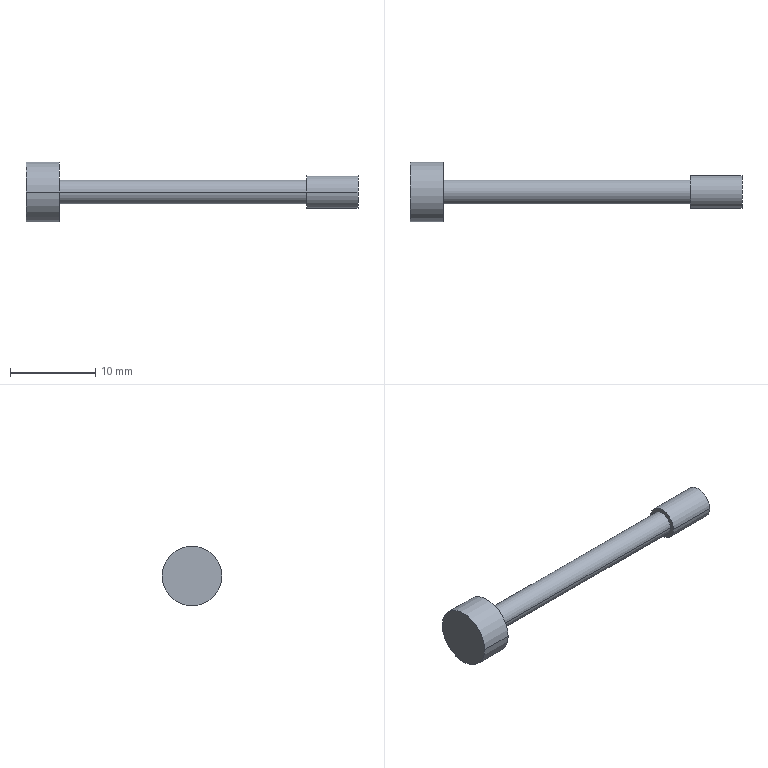Part | SolidWorks | features Revolution 1 | 1 solid | 10 faces | box 38.91 x 7 x 7 mm | volume 397.089 mm3 | cylinder 6 | plane 4 | commonest cylinder face diameters 2.8 x2 3.8 x2 7 x2
STEP:
#1=CARTESIAN_POINT('',(32.91,1.9,0.));
#2=VERTEX_POINT('',#1);
#3=CARTESIAN_POINT('',(32.91,-1.9,0.));
#4=VERTEX_POINT('',#3);
#5=CARTESIAN_POINT('',(32.91,0.,0.));
#6=DIRECTION('',(1.,0.,0.));
#7=DIRECTION('',(0.,1.,0.));
#8=AXIS2_PLACEMENT_3D('',#5,#6,#7);
#9=CIRCLE('',#8,1.9);
#10=EDGE_CURVE('',#2,#4,#9,.T.);
#11=ORIENTED_EDGE('',*,*,#10,.T.);
#12=CARTESIAN_POINT('',(38.91,-1.9,0.));
#13=VERTEX_POINT('',#12);
#14=CARTESIAN_POINT('',(38.91,-1.9,0.));
#15=DIRECTION('',(1.,0.,0.));
#16=VECTOR('',#15,1000.);
#17=LINE('',#14,#16);
#18=EDGE_CURVE('',#4,#13,#17,.T.);
#19=ORIENTED_EDGE('',*,*,#18,.T.);
#20=CARTESIAN_POINT('',(38.91,1.9,0.));
#21=VERTEX_POINT('',#20);
#22=CARTESIAN_POINT('',(38.91,0.,0.));
#23=DIRECTION('',(1.,0.,0.));
#24=DIRECTION('',(0.,1.,0.));
#25=AXIS2_PLACEMENT_3D('',#22,#23,#24);
#26=CIRCLE('',#25,1.9);
#27=EDGE_CURVE('',#21,#13,#26,.T.);
#28=ORIENTED_EDGE('',*,*,#27,.F.);
#29=CARTESIAN_POINT('',(38.91,1.9,0.));
#30=DIRECTION('',(1.,0.,0.));
#31=VECTOR('',#30,1000.);
#32=LINE('',#29,#31);
#33=EDGE_CURVE('',#2,#21,#32,.T.);
#34=ORIENTED_EDGE('',*,*,#33,.F.);
#35=EDGE_LOOP('',(#11,#19,#28,#34));
#36=FACE_OUTER_BOUND('',#35,.T.);
#37=CARTESIAN_POINT('',(38.91,0.,0.));
#38=DIRECTION('',(1.,0.,0.));
#39=DIRECTION('',(0.,1.,0.));
#40=AXIS2_PLACEMENT_3D('',#37,#38,#39);
#41=CYLINDRICAL_SURFACE('',#40,1.9);
#42=ADVANCED_FACE('',(#36),#41,.T.);
#43=CARTESIAN_POINT('',(3.91,1.4,0.));
#44=VERTEX_POINT('',#43);
#45=CARTESIAN_POINT('',(3.91,-1.4,0.));
#46=VERTEX_POINT('',#45);
#47=CARTESIAN_POINT('',(3.91,0.,0.));
#48=DIRECTION('',(1.,0.,0.));
#49=DIRECTION('',(0.,1.,0.));
#50=AXIS2_PLACEMENT_3D('',#47,#48,#49);
#51=CIRCLE('',#50,1.4);
#52=EDGE_CURVE('',#44,#46,#51,.T.);
#53=ORIENTED_EDGE('',*,*,#52,.T.);
#54=CARTESIAN_POINT('',(32.91,-1.4,0.));
#55=VERTEX_POINT('',#54);
#56=CARTESIAN_POINT('',(38.91,-1.4,0.));
#57=DIRECTION('',(1.,0.,0.));
#58=VECTOR('',#57,1000.);
#59=LINE('',#56,#58);
#60=EDGE_CURVE('',#46,#55,#59,.T.);
#61=ORIENTED_EDGE('',*,*,#60,.T.);
#62=CARTESIAN_POINT('',(32.91,1.4,0.));
#63=VERTEX_POINT('',#62);
#64=CARTESIAN_POINT('',(32.91,0.,0.));
#65=DIRECTION('',(1.,0.,0.));
#66=DIRECTION('',(0.,1.,0.));
#67=AXIS2_PLACEMENT_3D('',#64,#65,#66);
#68=CIRCLE('',#67,1.4);
#69=EDGE_CURVE('',#63,#55,#68,.T.);
#70=ORIENTED_EDGE('',*,*,#69,.F.);
#71=CARTESIAN_POINT('',(38.91,1.4,0.));
#72=DIRECTION('',(1.,0.,0.));
#73=VECTOR('',#72,1000.);
#74=LINE('',#71,#73);
#75=EDGE_CURVE('',#44,#63,#74,.T.);
#76=ORIENTED_EDGE('',*,*,#75,.F.);
#77=EDGE_LOOP('',(#53,#61,#70,#76));
#78=FACE_OUTER_BOUND('',#77,.T.);
#79=CARTESIAN_POINT('',(38.91,0.,0.));
#80=DIRECTION('',(1.,0.,0.));
#81=DIRECTION('',(0.,1.,0.));
#82=AXIS2_PLACEMENT_3D('',#79,#80,#81);
#83=CYLINDRICAL_SURFACE('',#82,1.4);
#84=ADVANCED_FACE('',(#78),#83,.T.);
#85=CARTESIAN_POINT('',(0.,3.5,0.));
#86=VERTEX_POINT('',#85);
#87=CARTESIAN_POINT('',(0.,-3.5,0.));
#88=VERTEX_POINT('',#87);
#89=CARTESIAN_POINT('',(0.,0.,0.));
#90=DIRECTION('',(1.,0.,0.));
#91=DIRECTION('',(0.,1.,0.));
#92=AXIS2_PLACEMENT_3D('',#89,#90,#91);
#93=CIRCLE('',#92,3.5);
#94=EDGE_CURVE('',#86,#88,#93,.T.);
#95=ORIENTED_EDGE('',*,*,#94,.T.);
#96=CARTESIAN_POINT('',(3.91,-3.5,0.));
#97=VERTEX_POINT('',#96);
#98=CARTESIAN_POINT('',(38.91,-3.5,0.));
#99=DIRECTION('',(1.,0.,0.));
#100=VECTOR('',#99,1000.);
#101=LINE('',#98,#100);
#102=EDGE_CURVE('',#88,#97,#101,.T.);
#103=ORIENTED_EDGE('',*,*,#102,.T.);
#104=CARTESIAN_POINT('',(3.91,3.5,0.));
#105=VERTEX_POINT('',#104);
#106=CARTESIAN_POINT('',(3.91,0.,0.));
#107=DIRECTION('',(1.,0.,0.));
#108=DIRECTION('',(0.,1.,0.));
#109=AXIS2_PLACEMENT_3D('',#106,#107,#108);
#110=CIRCLE('',#109,3.5);
#111=EDGE_CURVE('',#105,#97,#110,.T.);
#112=ORIENTED_EDGE('',*,*,#111,.F.);
#113=CARTESIAN_POINT('',(38.91,3.5,0.));
#114=DIRECTION('',(1.,0.,0.));
#115=VECTOR('',#114,1000.);
#116=LINE('',#113,#115);
#117=EDGE_CURVE('',#86,#105,#116,.T.);
#118=ORIENTED_EDGE('',*,*,#117,.F.);
#119=EDGE_LOOP('',(#95,#103,#112,#118));
#120=FACE_OUTER_BOUND('',#119,.T.);
#121=CARTESIAN_POINT('',(38.91,0.,0.));
#122=DIRECTION('',(1.,0.,0.));
#123=DIRECTION('',(0.,1.,0.));
#124=AXIS2_PLACEMENT_3D('',#121,#122,#123);
#125=CYLINDRICAL_SURFACE('',#124,3.5);
#126=ADVANCED_FACE('',(#120),#125,.T.);
#127=ORIENTED_EDGE('',*,*,#94,.F.);
#128=CARTESIAN_POINT('',(0.,0.,0.));
#129=DIRECTION('',(1.,0.,0.));
#130=DIRECTION('',(0.,1.,0.));
#131=AXIS2_PLACEMENT_3D('',#128,#129,#130);
#132=CIRCLE('',#131,3.5);
#133=EDGE_CURVE('',#88,#86,#132,.T.);
#134=ORIENTED_EDGE('',*,*,#133,.F.);
#135=EDGE_LOOP('',(#127,#134));
#136=FACE_OUTER_BOUND('',#135,.T.);
#137=CARTESIAN_POINT('',(0.,0.,0.));
#138=DIRECTION('',(-1.,0.,0.));
#139=DIRECTION('',(0.,-1.,0.));
#140=AXIS2_PLACEMENT_3D('',#137,#138,#139);
#141=PLANE('',#140);
#142=ADVANCED_FACE('',(#136),#141,.T.);
#143=ORIENTED_EDGE('',*,*,#102,.F.);
#144=ORIENTED_EDGE('',*,*,#133,.T.);
#145=ORIENTED_EDGE('',*,*,#117,.T.);
#146=CARTESIAN_POINT('',(3.91,0.,0.));
#147=DIRECTION('',(1.,0.,0.));
#148=DIRECTION('',(0.,1.,0.));
#149=AXIS2_PLACEMENT_3D('',#146,#147,#148);
#150=CIRCLE('',#149,3.5);
#151=EDGE_CURVE('',#97,#105,#150,.T.);
#152=ORIENTED_EDGE('',*,*,#151,.F.);
#153=EDGE_LOOP('',(#143,#144,#145,#152));
#154=FACE_OUTER_BOUND('',#153,.T.);
#155=CARTESIAN_POINT('',(38.91,0.,0.));
#156=DIRECTION('',(1.,0.,0.));
#157=DIRECTION('',(0.,1.,0.));
#158=AXIS2_PLACEMENT_3D('',#155,#156,#157);
#159=CYLINDRICAL_SURFACE('',#158,3.5);
#160=ADVANCED_FACE('',(#154),#159,.T.);
#161=ORIENTED_EDGE('',*,*,#111,.T.);
#162=ORIENTED_EDGE('',*,*,#151,.T.);
#163=EDGE_LOOP('',(#161,#162));
#164=FACE_OUTER_BOUND('',#163,.T.);
#165=ORIENTED_EDGE('',*,*,#52,.F.);
#166=CARTESIAN_POINT('',(3.91,0.,0.));
#167=DIRECTION('',(1.,0.,0.));
#168=DIRECTION('',(0.,1.,0.));
#169=AXIS2_PLACEMENT_3D('',#166,#167,#168);
#170=CIRCLE('',#169,1.4);
#171=EDGE_CURVE('',#46,#44,#170,.T.);
#172=ORIENTED_EDGE('',*,*,#171,.F.);
#173=EDGE_LOOP('',(#165,#172));
#174=FACE_BOUND('',#173,.T.);
#175=CARTESIAN_POINT('',(3.91,3.5,0.));
#176=DIRECTION('',(1.,0.,0.));
#177=DIRECTION('',(0.,1.,0.));
#178=AXIS2_PLACEMENT_3D('',#175,#176,#177);
#179=PLANE('',#178);
#180=ADVANCED_FACE('',(#164,#174),#179,.T.);
#181=ORIENTED_EDGE('',*,*,#60,.F.);
#182=ORIENTED_EDGE('',*,*,#171,.T.);
#183=ORIENTED_EDGE('',*,*,#75,.T.);
#184=CARTESIAN_POINT('',(32.91,0.,0.));
#185=DIRECTION('',(1.,0.,0.));
#186=DIRECTION('',(0.,1.,0.));
#187=AXIS2_PLACEMENT_3D('',#184,#185,#186);
#188=CIRCLE('',#187,1.4);
#189=EDGE_CURVE('',#55,#63,#188,.T.);
#190=ORIENTED_EDGE('',*,*,#189,.F.);
#191=EDGE_LOOP('',(#181,#182,#183,#190));
#192=FACE_OUTER_BOUND('',#191,.T.);
#193=CARTESIAN_POINT('',(38.91,0.,0.));
#194=DIRECTION('',(1.,0.,0.));
#195=DIRECTION('',(0.,1.,0.));
#196=AXIS2_PLACEMENT_3D('',#193,#194,#195);
#197=CYLINDRICAL_SURFACE('',#196,1.4);
#198=ADVANCED_FACE('',(#192),#197,.T.);
#199=ORIENTED_EDGE('',*,*,#69,.T.);
#200=ORIENTED_EDGE('',*,*,#189,.T.);
#201=EDGE_LOOP('',(#199,#200));
#202=FACE_BOUND('',#201,.T.);
#203=ORIENTED_EDGE('',*,*,#10,.F.);
#204=CARTESIAN_POINT('',(32.91,0.,0.));
#205=DIRECTION('',(1.,0.,0.));
#206=DIRECTION('',(0.,1.,0.));
#207=AXIS2_PLACEMENT_3D('',#204,#205,#206);
#208=CIRCLE('',#207,1.9);
#209=EDGE_CURVE('',#4,#2,#208,.T.);
#210=ORIENTED_EDGE('',*,*,#209,.F.);
#211=EDGE_LOOP('',(#203,#210));
#212=FACE_OUTER_BOUND('',#211,.T.);
#213=CARTESIAN_POINT('',(32.91,1.4,0.));
#214=DIRECTION('',(-1.,0.,0.));
#215=DIRECTION('',(0.,-1.,0.));
#216=AXIS2_PLACEMENT_3D('',#213,#214,#215);
#217=PLANE('',#216);
#218=ADVANCED_FACE('',(#202,#212),#217,.T.);
#219=ORIENTED_EDGE('',*,*,#18,.F.);
#220=ORIENTED_EDGE('',*,*,#209,.T.);
#221=ORIENTED_EDGE('',*,*,#33,.T.);
#222=CARTESIAN_POINT('',(38.91,0.,0.));
#223=DIRECTION('',(1.,0.,0.));
#224=DIRECTION('',(0.,1.,0.));
#225=AXIS2_PLACEMENT_3D('',#222,#223,#224);
#226=CIRCLE('',#225,1.9);
#227=EDGE_CURVE('',#13,#21,#226,.T.);
#228=ORIENTED_EDGE('',*,*,#227,.F.);
#229=EDGE_LOOP('',(#219,#220,#221,#228));
#230=FACE_OUTER_BOUND('',#229,.T.);
#231=CARTESIAN_POINT('',(38.91,0.,0.));
#232=DIRECTION('',(1.,0.,0.));
#233=DIRECTION('',(0.,1.,0.));
#234=AXIS2_PLACEMENT_3D('',#231,#232,#233);
#235=CYLINDRICAL_SURFACE('',#234,1.9);
#236=ADVANCED_FACE('',(#230),#235,.T.);
#237=ORIENTED_EDGE('',*,*,#27,.T.);
#238=ORIENTED_EDGE('',*,*,#227,.T.);
#239=EDGE_LOOP('',(#237,#238));
#240=FACE_OUTER_BOUND('',#239,.T.);
#241=CARTESIAN_POINT('',(38.91,0.,0.));
#242=DIRECTION('',(1.,0.,0.));
#243=DIRECTION('',(0.,1.,0.));
#244=AXIS2_PLACEMENT_3D('',#241,#242,#243);
#245=PLANE('',#244);
#246=ADVANCED_FACE('',(#240),#245,.T.);
#247=CLOSED_SHELL('',(#42,#84,#126,#142,#160,#180,#198,#218,#236,#246));
#248=MANIFOLD_SOLID_BREP('',#247);
#249=CARTESIAN_POINT('',(0.,0.,0.));
#250=DIRECTION('',(0.,0.,1.));
#251=DIRECTION('',(1.,0.,0.));
#252=AXIS2_PLACEMENT_3D('',#249,#250,#251);
#253=(LENGTH_UNIT()NAMED_UNIT(*)SI_UNIT(.MILLI.,.METRE.));
#254=UNCERTAINTY_MEASURE_WITH_UNIT(LENGTH_MEASURE(0.00001),#253,'','');
#255=(NAMED_UNIT(*)PLANE_ANGLE_UNIT()SI_UNIT($,.RADIAN.));
#256=(NAMED_UNIT(*)SI_UNIT($,.STERADIAN.)SOLID_ANGLE_UNIT());
#257=(GEOMETRIC_REPRESENTATION_CONTEXT(3)GLOBAL_UNCERTAINTY_ASSIGNED_CONTEXT((#254))GLOBAL_UNIT_ASSIGNED_CONTEXT((#253,#255,#256))REPRESENTATION_CONTEXT('',''));
#258=ADVANCED_BREP_SHAPE_REPRESENTATION('',(#248,#252),#257);